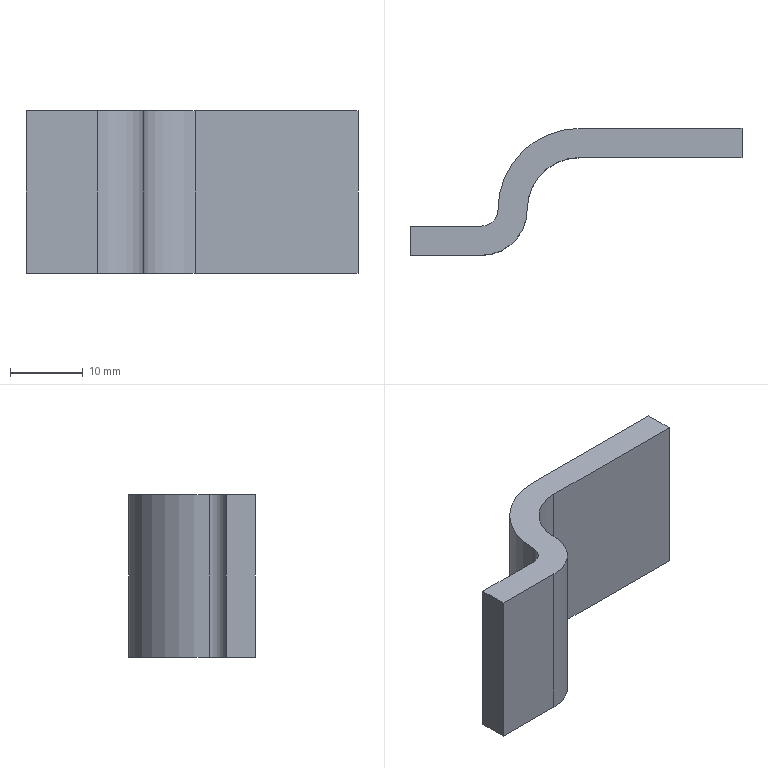Part | SolidWorks | features Extrusion 1 | 1 solid | 12 faces | box 45.542 x 17.392 x 22.352 mm | volume 4755 mm3 | plane 8 | cylinder 4 | commonest cylinder face diameters 4.56 x1 12.56 x1 14.224 x1 22.224 x1
STEP:
#1=CARTESIAN_POINT('',(0.,11.112,0.));
#2=VERTEX_POINT('',#1);
#3=CARTESIAN_POINT('',(-11.112,0.,0.));
#4=VERTEX_POINT('',#3);
#5=CARTESIAN_POINT('',(0.,0.,0.));
#6=DIRECTION('',(0.,0.,1.));
#7=DIRECTION('',(1.,0.,0.));
#8=AXIS2_PLACEMENT_3D('',#5,#6,#7);
#9=CIRCLE('',#8,11.112);
#10=EDGE_CURVE('',#2,#4,#9,.T.);
#11=ORIENTED_EDGE('',*,*,#10,.T.);
#12=CARTESIAN_POINT('',(-11.112,0.,22.352));
#13=VERTEX_POINT('',#12);
#14=CARTESIAN_POINT('',(-11.112,0.,22.352));
#15=DIRECTION('',(0.,0.,-1.));
#16=VECTOR('',#15,1000.);
#17=LINE('',#14,#16);
#18=EDGE_CURVE('',#13,#4,#17,.T.);
#19=ORIENTED_EDGE('',*,*,#18,.F.);
#20=CARTESIAN_POINT('',(0.,11.112,22.352));
#21=VERTEX_POINT('',#20);
#22=CARTESIAN_POINT('',(0.,0.,22.352));
#23=DIRECTION('',(0.,0.,1.));
#24=DIRECTION('',(1.,0.,0.));
#25=AXIS2_PLACEMENT_3D('',#22,#23,#24);
#26=CIRCLE('',#25,11.112);
#27=EDGE_CURVE('',#21,#13,#26,.T.);
#28=ORIENTED_EDGE('',*,*,#27,.F.);
#29=CARTESIAN_POINT('',(0.,11.112,22.352));
#30=DIRECTION('',(0.,0.,-1.));
#31=VECTOR('',#30,1000.);
#32=LINE('',#29,#31);
#33=EDGE_CURVE('',#21,#2,#32,.T.);
#34=ORIENTED_EDGE('',*,*,#33,.T.);
#35=EDGE_LOOP('',(#11,#19,#28,#34));
#36=FACE_OUTER_BOUND('',#35,.T.);
#37=CARTESIAN_POINT('',(0.,0.,22.352));
#38=DIRECTION('',(0.,0.,-1.));
#39=DIRECTION('',(-1.,0.,0.));
#40=AXIS2_PLACEMENT_3D('',#37,#38,#39);
#41=CYLINDRICAL_SURFACE('',#40,11.112);
#42=ADVANCED_FACE('',(#36),#41,.T.);
#43=CARTESIAN_POINT('',(-13.392,-2.28,0.));
#44=VERTEX_POINT('',#43);
#45=CARTESIAN_POINT('',(-13.392,0.,0.));
#46=DIRECTION('',(0.,0.,-1.));
#47=DIRECTION('',(1.,0.,0.));
#48=AXIS2_PLACEMENT_3D('',#45,#46,#47);
#49=CIRCLE('',#48,2.28);
#50=EDGE_CURVE('',#4,#44,#49,.T.);
#51=ORIENTED_EDGE('',*,*,#50,.T.);
#52=CARTESIAN_POINT('',(-13.392,-2.28,22.352));
#53=VERTEX_POINT('',#52);
#54=CARTESIAN_POINT('',(-13.392,-2.28,22.352));
#55=DIRECTION('',(0.,0.,-1.));
#56=VECTOR('',#55,1000.);
#57=LINE('',#54,#56);
#58=EDGE_CURVE('',#53,#44,#57,.T.);
#59=ORIENTED_EDGE('',*,*,#58,.F.);
#60=CARTESIAN_POINT('',(-13.392,0.,22.352));
#61=DIRECTION('',(0.,0.,-1.));
#62=DIRECTION('',(1.,0.,0.));
#63=AXIS2_PLACEMENT_3D('',#60,#61,#62);
#64=CIRCLE('',#63,2.28);
#65=EDGE_CURVE('',#13,#53,#64,.T.);
#66=ORIENTED_EDGE('',*,*,#65,.F.);
#67=ORIENTED_EDGE('',*,*,#18,.T.);
#68=EDGE_LOOP('',(#51,#59,#66,#67));
#69=FACE_OUTER_BOUND('',#68,.T.);
#70=CARTESIAN_POINT('',(-13.392,0.,22.352));
#71=DIRECTION('',(0.,0.,-1.));
#72=DIRECTION('',(-1.,0.,0.));
#73=AXIS2_PLACEMENT_3D('',#70,#71,#72);
#74=CYLINDRICAL_SURFACE('',#73,2.28);
#75=ADVANCED_FACE('',(#69),#74,.F.);
#76=CARTESIAN_POINT('',(-23.192,-2.28,0.));
#77=VERTEX_POINT('',#76);
#78=CARTESIAN_POINT('',(-13.392,-2.28,0.));
#79=DIRECTION('',(-1.,0.,0.));
#80=VECTOR('',#79,1000.);
#81=LINE('',#78,#80);
#82=EDGE_CURVE('',#44,#77,#81,.T.);
#83=ORIENTED_EDGE('',*,*,#82,.T.);
#84=CARTESIAN_POINT('',(-23.192,-2.28,22.352));
#85=VERTEX_POINT('',#84);
#86=CARTESIAN_POINT('',(-23.192,-2.28,22.352));
#87=DIRECTION('',(0.,0.,-1.));
#88=VECTOR('',#87,1000.);
#89=LINE('',#86,#88);
#90=EDGE_CURVE('',#85,#77,#89,.T.);
#91=ORIENTED_EDGE('',*,*,#90,.F.);
#92=CARTESIAN_POINT('',(-13.392,-2.28,22.352));
#93=DIRECTION('',(-1.,0.,0.));
#94=VECTOR('',#93,1000.);
#95=LINE('',#92,#94);
#96=EDGE_CURVE('',#53,#85,#95,.T.);
#97=ORIENTED_EDGE('',*,*,#96,.F.);
#98=ORIENTED_EDGE('',*,*,#58,.T.);
#99=EDGE_LOOP('',(#83,#91,#97,#98));
#100=FACE_OUTER_BOUND('',#99,.T.);
#101=CARTESIAN_POINT('',(-13.392,-2.28,22.352));
#102=DIRECTION('',(0.,-1.,0.));
#103=DIRECTION('',(0.,0.,-1.));
#104=AXIS2_PLACEMENT_3D('',#101,#102,#103);
#105=PLANE('',#104);
#106=ADVANCED_FACE('',(#100),#105,.F.);
#107=CARTESIAN_POINT('',(-23.192,-6.28,0.));
#108=VERTEX_POINT('',#107);
#109=CARTESIAN_POINT('',(-23.192,-2.28,0.));
#110=DIRECTION('',(0.,-1.,0.));
#111=VECTOR('',#110,1000.);
#112=LINE('',#109,#111);
#113=EDGE_CURVE('',#77,#108,#112,.T.);
#114=ORIENTED_EDGE('',*,*,#113,.T.);
#115=CARTESIAN_POINT('',(-23.192,-6.28,22.352));
#116=VERTEX_POINT('',#115);
#117=CARTESIAN_POINT('',(-23.192,-6.28,22.352));
#118=DIRECTION('',(0.,0.,-1.));
#119=VECTOR('',#118,1000.);
#120=LINE('',#117,#119);
#121=EDGE_CURVE('',#116,#108,#120,.T.);
#122=ORIENTED_EDGE('',*,*,#121,.F.);
#123=CARTESIAN_POINT('',(-23.192,-2.28,22.352));
#124=DIRECTION('',(0.,-1.,0.));
#125=VECTOR('',#124,1000.);
#126=LINE('',#123,#125);
#127=EDGE_CURVE('',#85,#116,#126,.T.);
#128=ORIENTED_EDGE('',*,*,#127,.F.);
#129=ORIENTED_EDGE('',*,*,#90,.T.);
#130=EDGE_LOOP('',(#114,#122,#128,#129));
#131=FACE_OUTER_BOUND('',#130,.T.);
#132=CARTESIAN_POINT('',(-23.192,-2.28,22.352));
#133=DIRECTION('',(1.,0.,0.));
#134=DIRECTION('',(0.,0.,-1.));
#135=AXIS2_PLACEMENT_3D('',#132,#133,#134);
#136=PLANE('',#135);
#137=ADVANCED_FACE('',(#131),#136,.F.);
#138=CARTESIAN_POINT('',(-13.392,-6.28,0.));
#139=VERTEX_POINT('',#138);
#140=CARTESIAN_POINT('',(-13.392,-6.28,0.));
#141=DIRECTION('',(1.,0.,0.));
#142=VECTOR('',#141,1000.);
#143=LINE('',#140,#142);
#144=EDGE_CURVE('',#108,#139,#143,.T.);
#145=ORIENTED_EDGE('',*,*,#144,.T.);
#146=CARTESIAN_POINT('',(-13.392,-6.28,22.352));
#147=VERTEX_POINT('',#146);
#148=CARTESIAN_POINT('',(-13.392,-6.28,22.352));
#149=DIRECTION('',(0.,0.,-1.));
#150=VECTOR('',#149,1000.);
#151=LINE('',#148,#150);
#152=EDGE_CURVE('',#147,#139,#151,.T.);
#153=ORIENTED_EDGE('',*,*,#152,.F.);
#154=CARTESIAN_POINT('',(-13.392,-6.28,22.352));
#155=DIRECTION('',(1.,0.,0.));
#156=VECTOR('',#155,1000.);
#157=LINE('',#154,#156);
#158=EDGE_CURVE('',#116,#147,#157,.T.);
#159=ORIENTED_EDGE('',*,*,#158,.F.);
#160=ORIENTED_EDGE('',*,*,#121,.T.);
#161=EDGE_LOOP('',(#145,#153,#159,#160));
#162=FACE_OUTER_BOUND('',#161,.T.);
#163=CARTESIAN_POINT('',(-13.392,-6.28,22.352));
#164=DIRECTION('',(0.,1.,0.));
#165=DIRECTION('',(0.,0.,1.));
#166=AXIS2_PLACEMENT_3D('',#163,#164,#165);
#167=PLANE('',#166);
#168=ADVANCED_FACE('',(#162),#167,.F.);
#169=CARTESIAN_POINT('',(-7.112,0.,0.));
#170=VERTEX_POINT('',#169);
#171=CARTESIAN_POINT('',(-13.392,0.,0.));
#172=DIRECTION('',(0.,0.,1.));
#173=DIRECTION('',(1.,0.,0.));
#174=AXIS2_PLACEMENT_3D('',#171,#172,#173);
#175=CIRCLE('',#174,6.28);
#176=EDGE_CURVE('',#139,#170,#175,.T.);
#177=ORIENTED_EDGE('',*,*,#176,.T.);
#178=CARTESIAN_POINT('',(-7.112,0.,22.352));
#179=VERTEX_POINT('',#178);
#180=CARTESIAN_POINT('',(-7.112,0.,22.352));
#181=DIRECTION('',(0.,0.,-1.));
#182=VECTOR('',#181,1000.);
#183=LINE('',#180,#182);
#184=EDGE_CURVE('',#179,#170,#183,.T.);
#185=ORIENTED_EDGE('',*,*,#184,.F.);
#186=CARTESIAN_POINT('',(-13.392,0.,22.352));
#187=DIRECTION('',(0.,0.,1.));
#188=DIRECTION('',(1.,0.,0.));
#189=AXIS2_PLACEMENT_3D('',#186,#187,#188);
#190=CIRCLE('',#189,6.28);
#191=EDGE_CURVE('',#147,#179,#190,.T.);
#192=ORIENTED_EDGE('',*,*,#191,.F.);
#193=ORIENTED_EDGE('',*,*,#152,.T.);
#194=EDGE_LOOP('',(#177,#185,#192,#193));
#195=FACE_OUTER_BOUND('',#194,.T.);
#196=CARTESIAN_POINT('',(-13.392,0.,22.352));
#197=DIRECTION('',(0.,0.,-1.));
#198=DIRECTION('',(-1.,0.,0.));
#199=AXIS2_PLACEMENT_3D('',#196,#197,#198);
#200=CYLINDRICAL_SURFACE('',#199,6.28);
#201=ADVANCED_FACE('',(#195),#200,.T.);
#202=CARTESIAN_POINT('',(0.,7.112,0.));
#203=VERTEX_POINT('',#202);
#204=CARTESIAN_POINT('',(0.,0.,0.));
#205=DIRECTION('',(0.,0.,-1.));
#206=DIRECTION('',(1.,0.,0.));
#207=AXIS2_PLACEMENT_3D('',#204,#205,#206);
#208=CIRCLE('',#207,7.112);
#209=EDGE_CURVE('',#170,#203,#208,.T.);
#210=ORIENTED_EDGE('',*,*,#209,.T.);
#211=CARTESIAN_POINT('',(0.,7.112,22.352));
#212=VERTEX_POINT('',#211);
#213=CARTESIAN_POINT('',(0.,7.112,22.352));
#214=DIRECTION('',(0.,0.,-1.));
#215=VECTOR('',#214,1000.);
#216=LINE('',#213,#215);
#217=EDGE_CURVE('',#212,#203,#216,.T.);
#218=ORIENTED_EDGE('',*,*,#217,.F.);
#219=CARTESIAN_POINT('',(0.,0.,22.352));
#220=DIRECTION('',(0.,0.,-1.));
#221=DIRECTION('',(1.,0.,0.));
#222=AXIS2_PLACEMENT_3D('',#219,#220,#221);
#223=CIRCLE('',#222,7.112);
#224=EDGE_CURVE('',#179,#212,#223,.T.);
#225=ORIENTED_EDGE('',*,*,#224,.F.);
#226=ORIENTED_EDGE('',*,*,#184,.T.);
#227=EDGE_LOOP('',(#210,#218,#225,#226));
#228=FACE_OUTER_BOUND('',#227,.T.);
#229=CARTESIAN_POINT('',(0.,0.,22.352));
#230=DIRECTION('',(0.,0.,-1.));
#231=DIRECTION('',(-1.,0.,0.));
#232=AXIS2_PLACEMENT_3D('',#229,#230,#231);
#233=CYLINDRICAL_SURFACE('',#232,7.112);
#234=ADVANCED_FACE('',(#228),#233,.F.);
#235=CARTESIAN_POINT('',(22.35,7.112,0.));
#236=VERTEX_POINT('',#235);
#237=CARTESIAN_POINT('',(0.,7.112,0.));
#238=DIRECTION('',(1.,0.,0.));
#239=VECTOR('',#238,1000.);
#240=LINE('',#237,#239);
#241=EDGE_CURVE('',#203,#236,#240,.T.);
#242=ORIENTED_EDGE('',*,*,#241,.T.);
#243=CARTESIAN_POINT('',(22.35,7.112,22.352));
#244=VERTEX_POINT('',#243);
#245=CARTESIAN_POINT('',(22.35,7.112,22.352));
#246=DIRECTION('',(0.,0.,-1.));
#247=VECTOR('',#246,1000.);
#248=LINE('',#245,#247);
#249=EDGE_CURVE('',#244,#236,#248,.T.);
#250=ORIENTED_EDGE('',*,*,#249,.F.);
#251=CARTESIAN_POINT('',(0.,7.112,22.352));
#252=DIRECTION('',(1.,0.,0.));
#253=VECTOR('',#252,1000.);
#254=LINE('',#251,#253);
#255=EDGE_CURVE('',#212,#244,#254,.T.);
#256=ORIENTED_EDGE('',*,*,#255,.F.);
#257=ORIENTED_EDGE('',*,*,#217,.T.);
#258=EDGE_LOOP('',(#242,#250,#256,#257));
#259=FACE_OUTER_BOUND('',#258,.T.);
#260=CARTESIAN_POINT('',(0.,7.112,22.352));
#261=DIRECTION('',(0.,1.,0.));
#262=DIRECTION('',(0.,0.,1.));
#263=AXIS2_PLACEMENT_3D('',#260,#261,#262);
#264=PLANE('',#263);
#265=ADVANCED_FACE('',(#259),#264,.F.);
#266=CARTESIAN_POINT('',(22.35,11.112,0.));
#267=VERTEX_POINT('',#266);
#268=CARTESIAN_POINT('',(22.35,11.112,0.));
#269=DIRECTION('',(0.,1.,0.));
#270=VECTOR('',#269,1000.);
#271=LINE('',#268,#270);
#272=EDGE_CURVE('',#236,#267,#271,.T.);
#273=ORIENTED_EDGE('',*,*,#272,.T.);
#274=CARTESIAN_POINT('',(22.35,11.112,22.352));
#275=VERTEX_POINT('',#274);
#276=CARTESIAN_POINT('',(22.35,11.112,22.352));
#277=DIRECTION('',(0.,0.,-1.));
#278=VECTOR('',#277,1000.);
#279=LINE('',#276,#278);
#280=EDGE_CURVE('',#275,#267,#279,.T.);
#281=ORIENTED_EDGE('',*,*,#280,.F.);
#282=CARTESIAN_POINT('',(22.35,11.112,22.352));
#283=DIRECTION('',(0.,1.,0.));
#284=VECTOR('',#283,1000.);
#285=LINE('',#282,#284);
#286=EDGE_CURVE('',#244,#275,#285,.T.);
#287=ORIENTED_EDGE('',*,*,#286,.F.);
#288=ORIENTED_EDGE('',*,*,#249,.T.);
#289=EDGE_LOOP('',(#273,#281,#287,#288));
#290=FACE_OUTER_BOUND('',#289,.T.);
#291=CARTESIAN_POINT('',(22.35,11.112,22.352));
#292=DIRECTION('',(-1.,0.,0.));
#293=DIRECTION('',(0.,0.,1.));
#294=AXIS2_PLACEMENT_3D('',#291,#292,#293);
#295=PLANE('',#294);
#296=ADVANCED_FACE('',(#290),#295,.F.);
#297=CARTESIAN_POINT('',(0.,11.112,0.));
#298=DIRECTION('',(-1.,0.,0.));
#299=VECTOR('',#298,1000.);
#300=LINE('',#297,#299);
#301=EDGE_CURVE('',#267,#2,#300,.T.);
#302=ORIENTED_EDGE('',*,*,#301,.T.);
#303=ORIENTED_EDGE('',*,*,#33,.F.);
#304=CARTESIAN_POINT('',(0.,11.112,22.352));
#305=DIRECTION('',(-1.,0.,0.));
#306=VECTOR('',#305,1000.);
#307=LINE('',#304,#306);
#308=EDGE_CURVE('',#275,#21,#307,.T.);
#309=ORIENTED_EDGE('',*,*,#308,.F.);
#310=ORIENTED_EDGE('',*,*,#280,.T.);
#311=EDGE_LOOP('',(#302,#303,#309,#310));
#312=FACE_OUTER_BOUND('',#311,.T.);
#313=CARTESIAN_POINT('',(0.,11.112,22.352));
#314=DIRECTION('',(0.,-1.,0.));
#315=DIRECTION('',(0.,0.,-1.));
#316=AXIS2_PLACEMENT_3D('',#313,#314,#315);
#317=PLANE('',#316);
#318=ADVANCED_FACE('',(#312),#317,.F.);
#319=ORIENTED_EDGE('',*,*,#27,.T.);
#320=ORIENTED_EDGE('',*,*,#65,.T.);
#321=ORIENTED_EDGE('',*,*,#96,.T.);
#322=ORIENTED_EDGE('',*,*,#127,.T.);
#323=ORIENTED_EDGE('',*,*,#158,.T.);
#324=ORIENTED_EDGE('',*,*,#191,.T.);
#325=ORIENTED_EDGE('',*,*,#224,.T.);
#326=ORIENTED_EDGE('',*,*,#255,.T.);
#327=ORIENTED_EDGE('',*,*,#286,.T.);
#328=ORIENTED_EDGE('',*,*,#308,.T.);
#329=EDGE_LOOP('',(#319,#320,#321,#322,#323,#324,#325,#326,#327,#328));
#330=FACE_OUTER_BOUND('',#329,.T.);
#331=CARTESIAN_POINT('',(0.,0.,22.352));
#332=DIRECTION('',(0.,0.,1.));
#333=DIRECTION('',(1.,0.,0.));
#334=AXIS2_PLACEMENT_3D('',#331,#332,#333);
#335=PLANE('',#334);
#336=ADVANCED_FACE('',(#330),#335,.T.);
#337=ORIENTED_EDGE('',*,*,#10,.F.);
#338=ORIENTED_EDGE('',*,*,#301,.F.);
#339=ORIENTED_EDGE('',*,*,#272,.F.);
#340=ORIENTED_EDGE('',*,*,#241,.F.);
#341=ORIENTED_EDGE('',*,*,#209,.F.);
#342=ORIENTED_EDGE('',*,*,#176,.F.);
#343=ORIENTED_EDGE('',*,*,#144,.F.);
#344=ORIENTED_EDGE('',*,*,#113,.F.);
#345=ORIENTED_EDGE('',*,*,#82,.F.);
#346=ORIENTED_EDGE('',*,*,#50,.F.);
#347=EDGE_LOOP('',(#337,#338,#339,#340,#341,#342,#343,#344,#345,#346));
#348=FACE_OUTER_BOUND('',#347,.T.);
#349=CARTESIAN_POINT('',(0.,0.,0.));
#350=DIRECTION('',(0.,0.,1.));
#351=DIRECTION('',(1.,0.,0.));
#352=AXIS2_PLACEMENT_3D('',#349,#350,#351);
#353=PLANE('',#352);
#354=ADVANCED_FACE('',(#348),#353,.F.);
#355=CLOSED_SHELL('',(#42,#75,#106,#137,#168,#201,#234,#265,#296,#318,#336,#354));
#356=MANIFOLD_SOLID_BREP('',#355);
#357=CARTESIAN_POINT('',(0.,0.,0.));
#358=DIRECTION('',(0.,0.,1.));
#359=DIRECTION('',(1.,0.,0.));
#360=AXIS2_PLACEMENT_3D('',#357,#358,#359);
#361=(LENGTH_UNIT()NAMED_UNIT(*)SI_UNIT(.MILLI.,.METRE.));
#362=UNCERTAINTY_MEASURE_WITH_UNIT(LENGTH_MEASURE(0.00001),#361,'','');
#363=(NAMED_UNIT(*)PLANE_ANGLE_UNIT()SI_UNIT($,.RADIAN.));
#364=(NAMED_UNIT(*)SI_UNIT($,.STERADIAN.)SOLID_ANGLE_UNIT());
#365=(GEOMETRIC_REPRESENTATION_CONTEXT(3)GLOBAL_UNCERTAINTY_ASSIGNED_CONTEXT((#362))GLOBAL_UNIT_ASSIGNED_CONTEXT((#361,#363,#364))REPRESENTATION_CONTEXT('',''));
#366=ADVANCED_BREP_SHAPE_REPRESENTATION('',(#356,#360),#365);